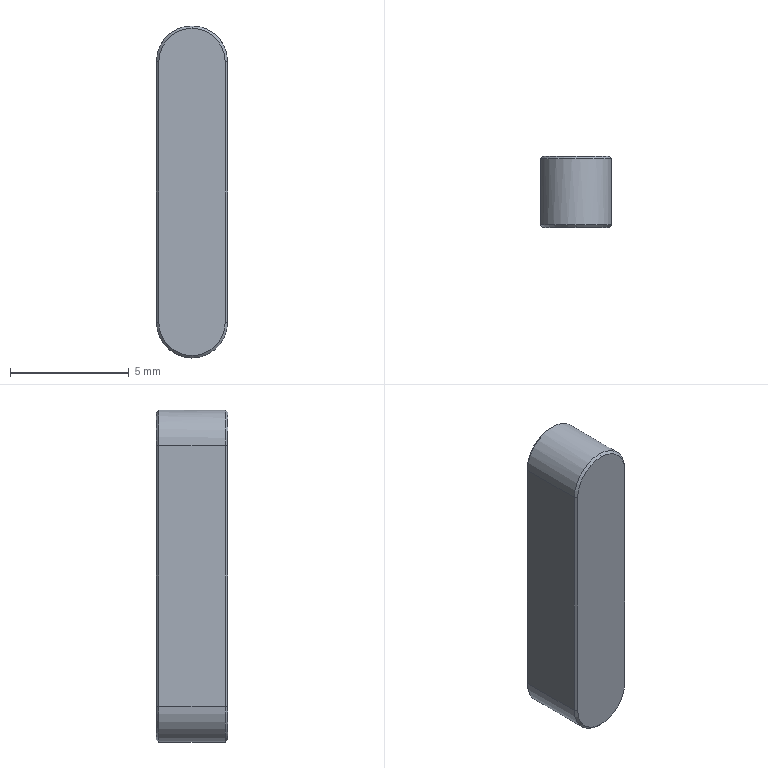Part | STEP file | 1 solid | 17 faces | box 3 x 3 x 14 mm | volume 119.894 mm3 | plane 8 | cone 6 | cylinder 3 | commonest cylinder face diameters 3 x3
STEP:
#1=CARTESIAN_POINT('',(0.,0.,0.));
#2=DIRECTION('',(0.,0.,1.));
#3=DIRECTION('',(1.,0.,0.));
#4=AXIS2_PLACEMENT_3D('',#1,#2,#3);
#5=CARTESIAN_POINT('',(0.,1.5,-6.9));
#6=VERTEX_POINT('',#5);
#7=CARTESIAN_POINT('',(-1.4,1.5,-5.5));
#8=VERTEX_POINT('',#7);
#9=CARTESIAN_POINT('',(0.,1.5,-5.5));
#10=DIRECTION('',(0.,1.,0.));
#11=DIRECTION('',(0.,0.,1.));
#12=AXIS2_PLACEMENT_3D('',#9,#10,#11);
#13=CIRCLE('',#12,1.4);
#14=CARTESIAN_POINT('',(0.,1.5,-5.5));
#15=DIRECTION('',(0.,-1.,0.));
#16=DIRECTION('',(0.,0.,-1.));
#17=AXIS2_PLACEMENT_3D('',#14,#15,#16);
#18=CONICAL_SURFACE('',#17,1.4,0.7854);
#19=CARTESIAN_POINT('',(9.425,0.));
#20=DIRECTION('',(-1.,0.));
#21=VECTOR('',#20,1.);
#22=LINE('',#19,#21);
#23=(GEOMETRIC_REPRESENTATION_CONTEXT(2)PARAMETRIC_REPRESENTATION_CONTEXT()REPRESENTATION_CONTEXT('',''));
#24=DEFINITIONAL_REPRESENTATION('',(#22),#23);
#25=PCURVE('',#18,#24);
#26=CARTESIAN_POINT('',(0.,1.5,5.5));
#27=DIRECTION('',(0.,1.,0.));
#28=DIRECTION('',(0.,0.,1.));
#29=AXIS2_PLACEMENT_3D('',#26,#27,#28);
#30=PLANE('',#29);
#31=CARTESIAN_POINT('',(-11.,0.));
#32=DIRECTION('',(1.,0.));
#33=AXIS2_PLACEMENT_2D('',#31,#32);
#34=CIRCLE('',#33,1.4);
#35=(GEOMETRIC_REPRESENTATION_CONTEXT(2)PARAMETRIC_REPRESENTATION_CONTEXT()REPRESENTATION_CONTEXT('',''));
#36=DEFINITIONAL_REPRESENTATION('',(#34),#35);
#37=PCURVE('',#30,#36);
#38=SURFACE_CURVE('',#13,(#25,#37),.PCURVE_S1.);
#39=EDGE_CURVE('',#6,#8,#38,.T.);
#40=ORIENTED_EDGE('',*,*,#39,.F.);
#41=CARTESIAN_POINT('',(0.,1.4,-7.));
#42=VERTEX_POINT('',#41);
#43=CARTESIAN_POINT('',(0.,1.5,-6.9));
#44=DIRECTION('',(0.,-0.7071,-0.7071));
#45=VECTOR('',#44,1.);
#46=LINE('',#43,#45);
#47=CARTESIAN_POINT('',(6.283,0.));
#48=DIRECTION('',(0.,1.));
#49=VECTOR('',#48,1.);
#50=LINE('',#47,#49);
#51=(GEOMETRIC_REPRESENTATION_CONTEXT(2)PARAMETRIC_REPRESENTATION_CONTEXT()REPRESENTATION_CONTEXT('',''));
#52=DEFINITIONAL_REPRESENTATION('',(#50),#51);
#53=PCURVE('',#18,#52);
#54=CARTESIAN_POINT('',(0.,1.5,-5.5));
#55=DIRECTION('',(0.,-1.,0.));
#56=DIRECTION('',(0.,0.,-1.));
#57=AXIS2_PLACEMENT_3D('',#54,#55,#56);
#58=CONICAL_SURFACE('',#57,1.4,0.7854);
#59=CARTESIAN_POINT('',(0.,0.));
#60=DIRECTION('',(0.,1.));
#61=VECTOR('',#60,1.);
#62=LINE('',#59,#61);
#63=(GEOMETRIC_REPRESENTATION_CONTEXT(2)PARAMETRIC_REPRESENTATION_CONTEXT()REPRESENTATION_CONTEXT('',''));
#64=DEFINITIONAL_REPRESENTATION('',(#62),#63);
#65=PCURVE('',#58,#64);
#66=SURFACE_CURVE('',#46,(#53,#65),.PCURVE_S1.);
#67=EDGE_CURVE('',#6,#42,#66,.T.);
#68=ORIENTED_EDGE('',*,*,#67,.T.);
#69=CARTESIAN_POINT('',(-1.5,1.4,-5.5));
#70=VERTEX_POINT('',#69);
#71=CARTESIAN_POINT('',(0.,1.4,-5.5));
#72=DIRECTION('',(0.,-1.,0.));
#73=DIRECTION('',(0.,0.,1.));
#74=AXIS2_PLACEMENT_3D('',#71,#72,#73);
#75=CIRCLE('',#74,1.5);
#76=CARTESIAN_POINT('',(3.142,0.1));
#77=DIRECTION('',(1.,0.));
#78=VECTOR('',#77,1.);
#79=LINE('',#76,#78);
#80=(GEOMETRIC_REPRESENTATION_CONTEXT(2)PARAMETRIC_REPRESENTATION_CONTEXT()REPRESENTATION_CONTEXT('',''));
#81=DEFINITIONAL_REPRESENTATION('',(#79),#80);
#82=PCURVE('',#18,#81);
#83=CARTESIAN_POINT('',(0.,1.5,-5.5));
#84=DIRECTION('',(0.,-1.,0.));
#85=DIRECTION('',(0.,0.,-1.));
#86=AXIS2_PLACEMENT_3D('',#83,#84,#85);
#87=CYLINDRICAL_SURFACE('',#86,1.5);
#88=CARTESIAN_POINT('',(3.142,0.1));
#89=DIRECTION('',(1.,0.));
#90=VECTOR('',#89,1.);
#91=LINE('',#88,#90);
#92=(GEOMETRIC_REPRESENTATION_CONTEXT(2)PARAMETRIC_REPRESENTATION_CONTEXT()REPRESENTATION_CONTEXT('',''));
#93=DEFINITIONAL_REPRESENTATION('',(#91),#92);
#94=PCURVE('',#87,#93);
#95=SURFACE_CURVE('',#75,(#82,#94),.PCURVE_S1.);
#96=EDGE_CURVE('',#70,#42,#95,.T.);
#97=ORIENTED_EDGE('',*,*,#96,.F.);
#98=CARTESIAN_POINT('',(-1.4,1.5,-5.5));
#99=DIRECTION('',(-0.7071,-0.7071,0.));
#100=VECTOR('',#99,1.);
#101=LINE('',#98,#100);
#102=CARTESIAN_POINT('',(4.712,0.));
#103=DIRECTION('',(0.,1.));
#104=VECTOR('',#103,1.);
#105=LINE('',#102,#104);
#106=(GEOMETRIC_REPRESENTATION_CONTEXT(2)PARAMETRIC_REPRESENTATION_CONTEXT()REPRESENTATION_CONTEXT('',''));
#107=DEFINITIONAL_REPRESENTATION('',(#105),#106);
#108=PCURVE('',#18,#107);
#109=CARTESIAN_POINT('',(-1.4,1.5,5.5));
#110=DIRECTION('',(-0.7071,0.7071,0.));
#111=DIRECTION('',(0.,0.,-1.));
#112=AXIS2_PLACEMENT_3D('',#109,#110,#111);
#113=PLANE('',#112);
#114=CARTESIAN_POINT('',(11.,0.));
#115=DIRECTION('',(0.,1.));
#116=VECTOR('',#115,1.);
#117=LINE('',#114,#116);
#118=(GEOMETRIC_REPRESENTATION_CONTEXT(2)PARAMETRIC_REPRESENTATION_CONTEXT()REPRESENTATION_CONTEXT('',''));
#119=DEFINITIONAL_REPRESENTATION('',(#117),#118);
#120=PCURVE('',#113,#119);
#121=SURFACE_CURVE('',#101,(#108,#120),.PCURVE_S1.);
#122=EDGE_CURVE('',#8,#70,#121,.T.);
#123=ORIENTED_EDGE('',*,*,#122,.F.);
#124=EDGE_LOOP('',(#40,#68,#97,#123));
#125=FACE_BOUND('',#124,.T.);
#126=ADVANCED_FACE('',(#125),#18,.T.);
#127=CARTESIAN_POINT('',(0.,-1.5,6.9));
#128=VERTEX_POINT('',#127);
#129=CARTESIAN_POINT('',(-1.4,-1.5,5.5));
#130=VERTEX_POINT('',#129);
#131=CARTESIAN_POINT('',(0.,-1.5,5.5));
#132=DIRECTION('',(0.,-1.,0.));
#133=DIRECTION('',(0.,0.,1.));
#134=AXIS2_PLACEMENT_3D('',#131,#132,#133);
#135=CIRCLE('',#134,1.4);
#136=CARTESIAN_POINT('',(0.,-1.4,5.5));
#137=DIRECTION('',(0.,1.,0.));
#138=DIRECTION('',(0.,0.,1.));
#139=AXIS2_PLACEMENT_3D('',#136,#137,#138);
#140=CONICAL_SURFACE('',#139,1.5,0.7854);
#141=CARTESIAN_POINT('',(6.283,-0.1));
#142=DIRECTION('',(-1.,0.));
#143=VECTOR('',#142,1.);
#144=LINE('',#141,#143);
#145=(GEOMETRIC_REPRESENTATION_CONTEXT(2)PARAMETRIC_REPRESENTATION_CONTEXT()REPRESENTATION_CONTEXT('',''));
#146=DEFINITIONAL_REPRESENTATION('',(#144),#145);
#147=PCURVE('',#140,#146);
#148=CARTESIAN_POINT('',(0.,-1.5,5.5));
#149=DIRECTION('',(0.,1.,0.));
#150=DIRECTION('',(0.,0.,1.));
#151=AXIS2_PLACEMENT_3D('',#148,#149,#150);
#152=PLANE('',#151);
#153=CARTESIAN_POINT('',(1.4,0.));
#154=CARTESIAN_POINT('',(1.4,-2.425));
#155=CARTESIAN_POINT('',(-0.7,-1.212));
#156=CARTESIAN_POINT('',(-2.8,0.));
#157=CARTESIAN_POINT('',(-0.7,1.212));
#158=CARTESIAN_POINT('',(1.4,2.425));
#159=CARTESIAN_POINT('',(1.4,0.));
#160=(BOUNDED_CURVE()B_SPLINE_CURVE(2,(#153,#154,#155,#156,#157,#158,#159),.UNSPECIFIED.,.T.,.F.)B_SPLINE_CURVE_WITH_KNOTS((1,2,2,2,2,1),(-2.094,0.,2.094,4.189,6.283,8.378),.UNSPECIFIED.)CURVE()GEOMETRIC_REPRESENTATION_ITEM()RATIONAL_B_SPLINE_CURVE((1.,0.5,1.,0.5,1.,0.5,1.))REPRESENTATION_ITEM(''));
#161=(GEOMETRIC_REPRESENTATION_CONTEXT(2)PARAMETRIC_REPRESENTATION_CONTEXT()REPRESENTATION_CONTEXT('',''));
#162=DEFINITIONAL_REPRESENTATION('',(#160),#161);
#163=PCURVE('',#152,#162);
#164=SURFACE_CURVE('',#135,(#147,#163),.PCURVE_S1.);
#165=EDGE_CURVE('',#128,#130,#164,.T.);
#166=ORIENTED_EDGE('',*,*,#165,.F.);
#167=CARTESIAN_POINT('',(0.,-1.4,7.));
#168=VERTEX_POINT('',#167);
#169=CARTESIAN_POINT('',(0.,-1.4,7.));
#170=DIRECTION('',(0.,0.7071,0.7071));
#171=VECTOR('',#170,1.);
#172=LINE('',#169,#171);
#173=CARTESIAN_POINT('',(6.283,0.));
#174=DIRECTION('',(0.,1.));
#175=VECTOR('',#174,1.);
#176=LINE('',#173,#175);
#177=(GEOMETRIC_REPRESENTATION_CONTEXT(2)PARAMETRIC_REPRESENTATION_CONTEXT()REPRESENTATION_CONTEXT('',''));
#178=DEFINITIONAL_REPRESENTATION('',(#176),#177);
#179=PCURVE('',#140,#178);
#180=CARTESIAN_POINT('',(0.,-1.4,5.5));
#181=DIRECTION('',(0.,1.,0.));
#182=DIRECTION('',(0.,0.,1.));
#183=AXIS2_PLACEMENT_3D('',#180,#181,#182);
#184=CONICAL_SURFACE('',#183,1.5,0.7854);
#185=CARTESIAN_POINT('',(0.,0.));
#186=DIRECTION('',(0.,1.));
#187=VECTOR('',#186,1.);
#188=LINE('',#185,#187);
#189=(GEOMETRIC_REPRESENTATION_CONTEXT(2)PARAMETRIC_REPRESENTATION_CONTEXT()REPRESENTATION_CONTEXT('',''));
#190=DEFINITIONAL_REPRESENTATION('',(#188),#189);
#191=PCURVE('',#184,#190);
#192=SURFACE_CURVE('',#172,(#179,#191),.PCURVE_S1.);
#193=EDGE_CURVE('',#128,#168,#192,.T.);
#194=ORIENTED_EDGE('',*,*,#193,.T.);
#195=CARTESIAN_POINT('',(-1.5,-1.4,5.5));
#196=VERTEX_POINT('',#195);
#197=CARTESIAN_POINT('',(0.,-1.4,5.5));
#198=DIRECTION('',(0.,1.,0.));
#199=DIRECTION('',(0.,0.,1.));
#200=AXIS2_PLACEMENT_3D('',#197,#198,#199);
#201=CIRCLE('',#200,1.5);
#202=CARTESIAN_POINT('',(0.,0.));
#203=DIRECTION('',(1.,0.));
#204=VECTOR('',#203,1.);
#205=LINE('',#202,#204);
#206=(GEOMETRIC_REPRESENTATION_CONTEXT(2)PARAMETRIC_REPRESENTATION_CONTEXT()REPRESENTATION_CONTEXT('',''));
#207=DEFINITIONAL_REPRESENTATION('',(#205),#206);
#208=PCURVE('',#140,#207);
#209=CARTESIAN_POINT('',(0.,1.5,5.5));
#210=DIRECTION('',(0.,-1.,0.));
#211=DIRECTION('',(0.,0.,-1.));
#212=AXIS2_PLACEMENT_3D('',#209,#210,#211);
#213=CYLINDRICAL_SURFACE('',#212,1.5);
#214=CARTESIAN_POINT('',(9.425,2.9));
#215=DIRECTION('',(-1.,0.));
#216=VECTOR('',#215,1.);
#217=LINE('',#214,#216);
#218=(GEOMETRIC_REPRESENTATION_CONTEXT(2)PARAMETRIC_REPRESENTATION_CONTEXT()REPRESENTATION_CONTEXT('',''));
#219=DEFINITIONAL_REPRESENTATION('',(#217),#218);
#220=PCURVE('',#213,#219);
#221=SURFACE_CURVE('',#201,(#208,#220),.PCURVE_S1.);
#222=EDGE_CURVE('',#196,#168,#221,.T.);
#223=ORIENTED_EDGE('',*,*,#222,.F.);
#224=CARTESIAN_POINT('',(-1.4,-1.5,5.5));
#225=DIRECTION('',(-0.7071,0.7071,0.));
#226=VECTOR('',#225,1.);
#227=LINE('',#224,#226);
#228=CARTESIAN_POINT('',(4.712,-0.1));
#229=DIRECTION('',(0.,1.));
#230=VECTOR('',#229,1.);
#231=LINE('',#228,#230);
#232=(GEOMETRIC_REPRESENTATION_CONTEXT(2)PARAMETRIC_REPRESENTATION_CONTEXT()REPRESENTATION_CONTEXT('',''));
#233=DEFINITIONAL_REPRESENTATION('',(#231),#232);
#234=PCURVE('',#140,#233);
#235=CARTESIAN_POINT('',(-1.5,-1.4,5.5));
#236=DIRECTION('',(0.7071,0.7071,0.));
#237=DIRECTION('',(0.,0.,1.));
#238=AXIS2_PLACEMENT_3D('',#235,#236,#237);
#239=PLANE('',#238);
#240=CARTESIAN_POINT('',(0.,0.1414));
#241=DIRECTION('',(0.,-1.));
#242=VECTOR('',#241,1.);
#243=LINE('',#240,#242);
#244=(GEOMETRIC_REPRESENTATION_CONTEXT(2)PARAMETRIC_REPRESENTATION_CONTEXT()REPRESENTATION_CONTEXT('',''));
#245=DEFINITIONAL_REPRESENTATION('',(#243),#244);
#246=PCURVE('',#239,#245);
#247=SURFACE_CURVE('',#227,(#234,#246),.PCURVE_S1.);
#248=EDGE_CURVE('',#130,#196,#247,.T.);
#249=ORIENTED_EDGE('',*,*,#248,.F.);
#250=EDGE_LOOP('',(#166,#194,#223,#249));
#251=FACE_BOUND('',#250,.T.);
#252=ADVANCED_FACE('',(#251),#140,.T.);
#253=ORIENTED_EDGE('',*,*,#96,.T.);
#254=CARTESIAN_POINT('',(0.,-1.4,-7.));
#255=VERTEX_POINT('',#254);
#256=CARTESIAN_POINT('',(0.,1.5,-7.));
#257=DIRECTION('',(0.,-1.,0.));
#258=VECTOR('',#257,1.);
#259=LINE('',#256,#258);
#260=CARTESIAN_POINT('',(6.283,0.));
#261=DIRECTION('',(0.,1.));
#262=VECTOR('',#261,1.);
#263=LINE('',#260,#262);
#264=(GEOMETRIC_REPRESENTATION_CONTEXT(2)PARAMETRIC_REPRESENTATION_CONTEXT()REPRESENTATION_CONTEXT('',''));
#265=DEFINITIONAL_REPRESENTATION('',(#263),#264);
#266=PCURVE('',#87,#265);
#267=CARTESIAN_POINT('',(0.,1.5,-5.5));
#268=DIRECTION('',(0.,-1.,0.));
#269=DIRECTION('',(0.,0.,-1.));
#270=AXIS2_PLACEMENT_3D('',#267,#268,#269);
#271=CYLINDRICAL_SURFACE('',#270,1.5);
#272=CARTESIAN_POINT('',(0.,0.));
#273=DIRECTION('',(0.,1.));
#274=VECTOR('',#273,1.);
#275=LINE('',#272,#274);
#276=(GEOMETRIC_REPRESENTATION_CONTEXT(2)PARAMETRIC_REPRESENTATION_CONTEXT()REPRESENTATION_CONTEXT('',''));
#277=DEFINITIONAL_REPRESENTATION('',(#275),#276);
#278=PCURVE('',#271,#277);
#279=SURFACE_CURVE('',#259,(#266,#278),.PCURVE_S1.);
#280=EDGE_CURVE('',#42,#255,#279,.T.);
#281=ORIENTED_EDGE('',*,*,#280,.T.);
#282=CARTESIAN_POINT('',(-1.5,-1.4,-5.5));
#283=VERTEX_POINT('',#282);
#284=CARTESIAN_POINT('',(0.,-1.4,-5.5));
#285=DIRECTION('',(0.,1.,0.));
#286=DIRECTION('',(0.,0.,1.));
#287=AXIS2_PLACEMENT_3D('',#284,#285,#286);
#288=CIRCLE('',#287,1.5);
#289=CARTESIAN_POINT('',(9.425,2.9));
#290=DIRECTION('',(-1.,0.));
#291=VECTOR('',#290,1.);
#292=LINE('',#289,#291);
#293=(GEOMETRIC_REPRESENTATION_CONTEXT(2)PARAMETRIC_REPRESENTATION_CONTEXT()REPRESENTATION_CONTEXT('',''));
#294=DEFINITIONAL_REPRESENTATION('',(#292),#293);
#295=PCURVE('',#87,#294);
#296=CARTESIAN_POINT('',(0.,-1.4,-5.5));
#297=DIRECTION('',(0.,1.,0.));
#298=DIRECTION('',(0.,0.,1.));
#299=AXIS2_PLACEMENT_3D('',#296,#297,#298);
#300=CONICAL_SURFACE('',#299,1.5,0.7854);
#301=CARTESIAN_POINT('',(0.,0.));
#302=DIRECTION('',(1.,0.));
#303=VECTOR('',#302,1.);
#304=LINE('',#301,#303);
#305=(GEOMETRIC_REPRESENTATION_CONTEXT(2)PARAMETRIC_REPRESENTATION_CONTEXT()REPRESENTATION_CONTEXT('',''));
#306=DEFINITIONAL_REPRESENTATION('',(#304),#305);
#307=PCURVE('',#300,#306);
#308=SURFACE_CURVE('',#288,(#295,#307),.PCURVE_S1.);
#309=EDGE_CURVE('',#255,#283,#308,.T.);
#310=ORIENTED_EDGE('',*,*,#309,.T.);
#311=CARTESIAN_POINT('',(-1.5,1.5,-5.5));
#312=DIRECTION('',(0.,-1.,0.));
#313=VECTOR('',#312,1.);
#314=LINE('',#311,#313);
#315=CARTESIAN_POINT('',(4.712,0.));
#316=DIRECTION('',(0.,1.));
#317=VECTOR('',#316,1.);
#318=LINE('',#315,#317);
#319=(GEOMETRIC_REPRESENTATION_CONTEXT(2)PARAMETRIC_REPRESENTATION_CONTEXT()REPRESENTATION_CONTEXT('',''));
#320=DEFINITIONAL_REPRESENTATION('',(#318),#319);
#321=PCURVE('',#87,#320);
#322=CARTESIAN_POINT('',(-1.5,1.5,5.5));
#323=DIRECTION('',(1.,0.,0.));
#324=DIRECTION('',(0.,0.,-1.));
#325=AXIS2_PLACEMENT_3D('',#322,#323,#324);
#326=PLANE('',#325);
#327=CARTESIAN_POINT('',(11.,0.));
#328=DIRECTION('',(0.,-1.));
#329=VECTOR('',#328,1.);
#330=LINE('',#327,#329);
#331=(GEOMETRIC_REPRESENTATION_CONTEXT(2)PARAMETRIC_REPRESENTATION_CONTEXT()REPRESENTATION_CONTEXT('',''));
#332=DEFINITIONAL_REPRESENTATION('',(#330),#331);
#333=PCURVE('',#326,#332);
#334=SURFACE_CURVE('',#314,(#321,#333),.PCURVE_S1.);
#335=EDGE_CURVE('',#70,#283,#334,.T.);
#336=ORIENTED_EDGE('',*,*,#335,.F.);
#337=EDGE_LOOP('',(#253,#281,#310,#336));
#338=FACE_BOUND('',#337,.T.);
#339=ADVANCED_FACE('',(#338),#87,.T.);
#340=CARTESIAN_POINT('',(-1.5,1.4,5.5));
#341=VERTEX_POINT('',#340);
#342=CARTESIAN_POINT('',(-1.5,1.5,5.5));
#343=DIRECTION('',(0.,-1.,0.));
#344=VECTOR('',#343,1.);
#345=LINE('',#342,#344);
#346=CARTESIAN_POINT('',(4.712,0.));
#347=DIRECTION('',(0.,1.));
#348=VECTOR('',#347,1.);
#349=LINE('',#346,#348);
#350=(GEOMETRIC_REPRESENTATION_CONTEXT(2)PARAMETRIC_REPRESENTATION_CONTEXT()REPRESENTATION_CONTEXT('',''));
#351=DEFINITIONAL_REPRESENTATION('',(#349),#350);
#352=PCURVE('',#213,#351);
#353=CARTESIAN_POINT('',(0.,0.));
#354=DIRECTION('',(0.,-1.));
#355=VECTOR('',#354,1.);
#356=LINE('',#353,#355);
#357=(GEOMETRIC_REPRESENTATION_CONTEXT(2)PARAMETRIC_REPRESENTATION_CONTEXT()REPRESENTATION_CONTEXT('',''));
#358=DEFINITIONAL_REPRESENTATION('',(#356),#357);
#359=PCURVE('',#326,#358);
#360=SURFACE_CURVE('',#345,(#352,#359),.PCURVE_S1.);
#361=EDGE_CURVE('',#341,#196,#360,.T.);
#362=ORIENTED_EDGE('',*,*,#361,.T.);
#363=ORIENTED_EDGE('',*,*,#222,.T.);
#364=CARTESIAN_POINT('',(1.5,-1.4,5.5));
#365=VERTEX_POINT('',#364);
#366=CARTESIAN_POINT('',(0.,-1.4,5.5));
#367=DIRECTION('',(0.,1.,0.));
#368=DIRECTION('',(0.,0.,1.));
#369=AXIS2_PLACEMENT_3D('',#366,#367,#368);
#370=CIRCLE('',#369,1.5);
#371=CARTESIAN_POINT('',(3.142,2.9));
#372=DIRECTION('',(-1.,0.));
#373=VECTOR('',#372,1.);
#374=LINE('',#371,#373);
#375=(GEOMETRIC_REPRESENTATION_CONTEXT(2)PARAMETRIC_REPRESENTATION_CONTEXT()REPRESENTATION_CONTEXT('',''));
#376=DEFINITIONAL_REPRESENTATION('',(#374),#375);
#377=PCURVE('',#213,#376);
#378=CARTESIAN_POINT('',(0.,0.));
#379=DIRECTION('',(1.,0.));
#380=VECTOR('',#379,1.);
#381=LINE('',#378,#380);
#382=(GEOMETRIC_REPRESENTATION_CONTEXT(2)PARAMETRIC_REPRESENTATION_CONTEXT()REPRESENTATION_CONTEXT('',''));
#383=DEFINITIONAL_REPRESENTATION('',(#381),#382);
#384=PCURVE('',#184,#383);
#385=SURFACE_CURVE('',#370,(#377,#384),.PCURVE_S1.);
#386=EDGE_CURVE('',#168,#365,#385,.T.);
#387=ORIENTED_EDGE('',*,*,#386,.T.);
#388=CARTESIAN_POINT('',(1.5,1.4,5.5));
#389=VERTEX_POINT('',#388);
#390=CARTESIAN_POINT('',(1.5,1.5,5.5));
#391=DIRECTION('',(0.,-1.,0.));
#392=VECTOR('',#391,1.);
#393=LINE('',#390,#392);
#394=CARTESIAN_POINT('',(1.571,0.));
#395=DIRECTION('',(0.,1.));
#396=VECTOR('',#395,1.);
#397=LINE('',#394,#396);
#398=(GEOMETRIC_REPRESENTATION_CONTEXT(2)PARAMETRIC_REPRESENTATION_CONTEXT()REPRESENTATION_CONTEXT('',''));
#399=DEFINITIONAL_REPRESENTATION('',(#397),#398);
#400=PCURVE('',#213,#399);
#401=CARTESIAN_POINT('',(1.5,1.5,5.5));
#402=DIRECTION('',(-1.,0.,0.));
#403=DIRECTION('',(0.,0.,1.));
#404=AXIS2_PLACEMENT_3D('',#401,#402,#403);
#405=PLANE('',#404);
#406=CARTESIAN_POINT('',(0.,0.));
#407=DIRECTION('',(0.,-1.));
#408=VECTOR('',#407,1.);
#409=LINE('',#406,#408);
#410=(GEOMETRIC_REPRESENTATION_CONTEXT(2)PARAMETRIC_REPRESENTATION_CONTEXT()REPRESENTATION_CONTEXT('',''));
#411=DEFINITIONAL_REPRESENTATION('',(#409),#410);
#412=PCURVE('',#405,#411);
#413=SURFACE_CURVE('',#393,(#400,#412),.PCURVE_S1.);
#414=EDGE_CURVE('',#389,#365,#413,.T.);
#415=ORIENTED_EDGE('',*,*,#414,.F.);
#416=CARTESIAN_POINT('',(0.,1.4,5.5));
#417=DIRECTION('',(0.,-1.,0.));
#418=DIRECTION('',(0.,0.,1.));
#419=AXIS2_PLACEMENT_3D('',#416,#417,#418);
#420=CIRCLE('',#419,1.5);
#421=CARTESIAN_POINT('',(-3.142,0.1));
#422=DIRECTION('',(1.,0.));
#423=VECTOR('',#422,1.);
#424=LINE('',#421,#423);
#425=(GEOMETRIC_REPRESENTATION_CONTEXT(2)PARAMETRIC_REPRESENTATION_CONTEXT()REPRESENTATION_CONTEXT('',''));
#426=DEFINITIONAL_REPRESENTATION('',(#424),#425);
#427=PCURVE('',#213,#426);
#428=CARTESIAN_POINT('',(0.,1.5,5.5));
#429=DIRECTION('',(0.,-1.,0.));
#430=DIRECTION('',(0.,0.,-1.));
#431=AXIS2_PLACEMENT_3D('',#428,#429,#430);
#432=CONICAL_SURFACE('',#431,1.4,0.7854);
#433=CARTESIAN_POINT('',(-3.142,0.1));
#434=DIRECTION('',(1.,0.));
#435=VECTOR('',#434,1.);
#436=LINE('',#433,#435);
#437=(GEOMETRIC_REPRESENTATION_CONTEXT(2)PARAMETRIC_REPRESENTATION_CONTEXT()REPRESENTATION_CONTEXT('',''));
#438=DEFINITIONAL_REPRESENTATION('',(#436),#437);
#439=PCURVE('',#432,#438);
#440=SURFACE_CURVE('',#420,(#427,#439),.PCURVE_S1.);
#441=EDGE_CURVE('',#389,#341,#440,.T.);
#442=ORIENTED_EDGE('',*,*,#441,.T.);
#443=EDGE_LOOP('',(#362,#363,#387,#415,#442));
#444=FACE_BOUND('',#443,.T.);
#445=ADVANCED_FACE('',(#444),#213,.T.);
#446=ORIENTED_EDGE('',*,*,#414,.T.);
#447=CARTESIAN_POINT('',(1.5,-1.4,-5.5));
#448=VERTEX_POINT('',#447);
#449=CARTESIAN_POINT('',(1.5,-1.4,5.5));
#450=DIRECTION('',(0.,0.,-1.));
#451=VECTOR('',#450,1.);
#452=LINE('',#449,#451);
#453=CARTESIAN_POINT('',(0.,-2.9));
#454=DIRECTION('',(-1.,0.));
#455=VECTOR('',#454,1.);
#456=LINE('',#453,#455);
#457=(GEOMETRIC_REPRESENTATION_CONTEXT(2)PARAMETRIC_REPRESENTATION_CONTEXT()REPRESENTATION_CONTEXT('',''));
#458=DEFINITIONAL_REPRESENTATION('',(#456),#457);
#459=PCURVE('',#405,#458);
#460=CARTESIAN_POINT('',(1.5,-1.4,5.5));
#461=DIRECTION('',(-0.7071,0.7071,0.));
#462=DIRECTION('',(0.,0.,-1.));
#463=AXIS2_PLACEMENT_3D('',#460,#461,#462);
#464=PLANE('',#463);
#465=CARTESIAN_POINT('',(0.,0.));
#466=DIRECTION('',(1.,0.));
#467=VECTOR('',#466,1.);
#468=LINE('',#465,#467);
#469=(GEOMETRIC_REPRESENTATION_CONTEXT(2)PARAMETRIC_REPRESENTATION_CONTEXT()REPRESENTATION_CONTEXT('',''));
#470=DEFINITIONAL_REPRESENTATION('',(#468),#469);
#471=PCURVE('',#464,#470);
#472=SURFACE_CURVE('',#452,(#459,#471),.PCURVE_S1.);
#473=EDGE_CURVE('',#365,#448,#472,.T.);
#474=ORIENTED_EDGE('',*,*,#473,.T.);
#475=CARTESIAN_POINT('',(1.5,1.4,-5.5));
#476=VERTEX_POINT('',#475);
#477=CARTESIAN_POINT('',(1.5,1.5,-5.5));
#478=DIRECTION('',(0.,-1.,0.));
#479=VECTOR('',#478,1.);
#480=LINE('',#477,#479);
#481=CARTESIAN_POINT('',(-11.,0.));
#482=DIRECTION('',(0.,-1.));
#483=VECTOR('',#482,1.);
#484=LINE('',#481,#483);
#485=(GEOMETRIC_REPRESENTATION_CONTEXT(2)PARAMETRIC_REPRESENTATION_CONTEXT()REPRESENTATION_CONTEXT('',''));
#486=DEFINITIONAL_REPRESENTATION('',(#484),#485);
#487=PCURVE('',#405,#486);
#488=CARTESIAN_POINT('',(1.571,0.));
#489=DIRECTION('',(0.,1.));
#490=VECTOR('',#489,1.);
#491=LINE('',#488,#490);
#492=(GEOMETRIC_REPRESENTATION_CONTEXT(2)PARAMETRIC_REPRESENTATION_CONTEXT()REPRESENTATION_CONTEXT('',''));
#493=DEFINITIONAL_REPRESENTATION('',(#491),#492);
#494=PCURVE('',#271,#493);
#495=SURFACE_CURVE('',#480,(#487,#494),.PCURVE_S1.);
#496=EDGE_CURVE('',#476,#448,#495,.T.);
#497=ORIENTED_EDGE('',*,*,#496,.F.);
#498=CARTESIAN_POINT('',(1.5,1.4,5.5));
#499=DIRECTION('',(0.,0.,1.));
#500=VECTOR('',#499,1.);
#501=LINE('',#498,#500);
#502=CARTESIAN_POINT('',(0.,-0.1));
#503=DIRECTION('',(1.,0.));
#504=VECTOR('',#503,1.);
#505=LINE('',#502,#504);
#506=(GEOMETRIC_REPRESENTATION_CONTEXT(2)PARAMETRIC_REPRESENTATION_CONTEXT()REPRESENTATION_CONTEXT('',''));
#507=DEFINITIONAL_REPRESENTATION('',(#505),#506);
#508=PCURVE('',#405,#507);
#509=CARTESIAN_POINT('',(1.4,1.5,5.5));
#510=DIRECTION('',(0.7071,0.7071,0.));
#511=DIRECTION('',(0.,0.,1.));
#512=AXIS2_PLACEMENT_3D('',#509,#510,#511);
#513=PLANE('',#512);
#514=CARTESIAN_POINT('',(0.,0.1414));
#515=DIRECTION('',(1.,0.));
#516=VECTOR('',#515,1.);
#517=LINE('',#514,#516);
#518=(GEOMETRIC_REPRESENTATION_CONTEXT(2)PARAMETRIC_REPRESENTATION_CONTEXT()REPRESENTATION_CONTEXT('',''));
#519=DEFINITIONAL_REPRESENTATION('',(#517),#518);
#520=PCURVE('',#513,#519);
#521=SURFACE_CURVE('',#501,(#508,#520),.PCURVE_S1.);
#522=EDGE_CURVE('',#476,#389,#521,.T.);
#523=ORIENTED_EDGE('',*,*,#522,.T.);
#524=EDGE_LOOP('',(#446,#474,#497,#523));
#525=FACE_BOUND('',#524,.T.);
#526=ADVANCED_FACE('',(#525),#405,.F.);
#527=ORIENTED_EDGE('',*,*,#280,.F.);
#528=CARTESIAN_POINT('',(0.,1.4,-5.5));
#529=DIRECTION('',(0.,-1.,0.));
#530=DIRECTION('',(0.,0.,1.));
#531=AXIS2_PLACEMENT_3D('',#528,#529,#530);
#532=CIRCLE('',#531,1.5);
#533=CARTESIAN_POINT('',(-3.142,0.1));
#534=DIRECTION('',(1.,0.));
#535=VECTOR('',#534,1.);
#536=LINE('',#533,#535);
#537=(GEOMETRIC_REPRESENTATION_CONTEXT(2)PARAMETRIC_REPRESENTATION_CONTEXT()REPRESENTATION_CONTEXT('',''));
#538=DEFINITIONAL_REPRESENTATION('',(#536),#537);
#539=PCURVE('',#271,#538);
#540=CARTESIAN_POINT('',(-3.142,0.1));
#541=DIRECTION('',(1.,0.));
#542=VECTOR('',#541,1.);
#543=LINE('',#540,#542);
#544=(GEOMETRIC_REPRESENTATION_CONTEXT(2)PARAMETRIC_REPRESENTATION_CONTEXT()REPRESENTATION_CONTEXT('',''));
#545=DEFINITIONAL_REPRESENTATION('',(#543),#544);
#546=PCURVE('',#58,#545);
#547=SURFACE_CURVE('',#532,(#539,#546),.PCURVE_S1.);
#548=EDGE_CURVE('',#42,#476,#547,.T.);
#549=ORIENTED_EDGE('',*,*,#548,.T.);
#550=ORIENTED_EDGE('',*,*,#496,.T.);
#551=CARTESIAN_POINT('',(0.,-1.4,-5.5));
#552=DIRECTION('',(0.,1.,0.));
#553=DIRECTION('',(0.,0.,1.));
#554=AXIS2_PLACEMENT_3D('',#551,#552,#553);
#555=CIRCLE('',#554,1.5);
#556=CARTESIAN_POINT('',(3.142,2.9));
#557=DIRECTION('',(-1.,0.));
#558=VECTOR('',#557,1.);
#559=LINE('',#556,#558);
#560=(GEOMETRIC_REPRESENTATION_CONTEXT(2)PARAMETRIC_REPRESENTATION_CONTEXT()REPRESENTATION_CONTEXT('',''));
#561=DEFINITIONAL_REPRESENTATION('',(#559),#560);
#562=PCURVE('',#271,#561);
#563=CARTESIAN_POINT('',(0.,0.));
#564=DIRECTION('',(1.,0.));
#565=VECTOR('',#564,1.);
#566=LINE('',#563,#565);
#567=(GEOMETRIC_REPRESENTATION_CONTEXT(2)PARAMETRIC_REPRESENTATION_CONTEXT()REPRESENTATION_CONTEXT('',''));
#568=DEFINITIONAL_REPRESENTATION('',(#566),#567);
#569=PCURVE('',#300,#568);
#570=SURFACE_CURVE('',#555,(#562,#569),.PCURVE_S1.);
#571=EDGE_CURVE('',#448,#255,#570,.T.);
#572=ORIENTED_EDGE('',*,*,#571,.T.);
#573=EDGE_LOOP('',(#527,#549,#550,#572));
#574=FACE_BOUND('',#573,.T.);
#575=ADVANCED_FACE('',(#574),#271,.T.);
#576=ORIENTED_EDGE('',*,*,#335,.T.);
#577=CARTESIAN_POINT('',(-1.5,-1.4,5.5));
#578=DIRECTION('',(0.,0.,1.));
#579=VECTOR('',#578,1.);
#580=LINE('',#577,#579);
#581=CARTESIAN_POINT('',(0.,-2.9));
#582=DIRECTION('',(-1.,0.));
#583=VECTOR('',#582,1.);
#584=LINE('',#581,#583);
#585=(GEOMETRIC_REPRESENTATION_CONTEXT(2)PARAMETRIC_REPRESENTATION_CONTEXT()REPRESENTATION_CONTEXT('',''));
#586=DEFINITIONAL_REPRESENTATION('',(#584),#585);
#587=PCURVE('',#326,#586);
#588=CARTESIAN_POINT('',(0.,0.));
#589=DIRECTION('',(1.,0.));
#590=VECTOR('',#589,1.);
#591=LINE('',#588,#590);
#592=(GEOMETRIC_REPRESENTATION_CONTEXT(2)PARAMETRIC_REPRESENTATION_CONTEXT()REPRESENTATION_CONTEXT('',''));
#593=DEFINITIONAL_REPRESENTATION('',(#591),#592);
#594=PCURVE('',#239,#593);
#595=SURFACE_CURVE('',#580,(#587,#594),.PCURVE_S1.);
#596=EDGE_CURVE('',#283,#196,#595,.T.);
#597=ORIENTED_EDGE('',*,*,#596,.T.);
#598=ORIENTED_EDGE('',*,*,#361,.F.);
#599=CARTESIAN_POINT('',(-1.5,1.4,-5.5));
#600=DIRECTION('',(0.,0.,-1.));
#601=VECTOR('',#600,1.);
#602=LINE('',#599,#601);
#603=CARTESIAN_POINT('',(11.,-0.1));
#604=DIRECTION('',(1.,0.));
#605=VECTOR('',#604,1.);
#606=LINE('',#603,#605);
#607=(GEOMETRIC_REPRESENTATION_CONTEXT(2)PARAMETRIC_REPRESENTATION_CONTEXT()REPRESENTATION_CONTEXT('',''));
#608=DEFINITIONAL_REPRESENTATION('',(#606),#607);
#609=PCURVE('',#326,#608);
#610=CARTESIAN_POINT('',(11.,0.1414));
#611=DIRECTION('',(1.,0.));
#612=VECTOR('',#611,1.);
#613=LINE('',#610,#612);
#614=(GEOMETRIC_REPRESENTATION_CONTEXT(2)PARAMETRIC_REPRESENTATION_CONTEXT()REPRESENTATION_CONTEXT('',''));
#615=DEFINITIONAL_REPRESENTATION('',(#613),#614);
#616=PCURVE('',#113,#615);
#617=SURFACE_CURVE('',#602,(#609,#616),.PCURVE_S1.);
#618=EDGE_CURVE('',#341,#70,#617,.T.);
#619=ORIENTED_EDGE('',*,*,#618,.T.);
#620=EDGE_LOOP('',(#576,#597,#598,#619));
#621=FACE_BOUND('',#620,.T.);
#622=ADVANCED_FACE('',(#621),#326,.F.);
#623=CARTESIAN_POINT('',(1.4,1.5,-5.5));
#624=VERTEX_POINT('',#623);
#625=CARTESIAN_POINT('',(0.,1.5,-5.5));
#626=DIRECTION('',(0.,1.,0.));
#627=DIRECTION('',(0.,0.,1.));
#628=AXIS2_PLACEMENT_3D('',#625,#626,#627);
#629=CIRCLE('',#628,1.4);
#630=CARTESIAN_POINT('',(-11.,0.));
#631=DIRECTION('',(1.,0.));
#632=AXIS2_PLACEMENT_2D('',#630,#631);
#633=CIRCLE('',#632,1.4);
#634=(GEOMETRIC_REPRESENTATION_CONTEXT(2)PARAMETRIC_REPRESENTATION_CONTEXT()REPRESENTATION_CONTEXT('',''));
#635=DEFINITIONAL_REPRESENTATION('',(#633),#634);
#636=PCURVE('',#30,#635);
#637=CARTESIAN_POINT('',(3.142,0.));
#638=DIRECTION('',(-1.,0.));
#639=VECTOR('',#638,1.);
#640=LINE('',#637,#639);
#641=(GEOMETRIC_REPRESENTATION_CONTEXT(2)PARAMETRIC_REPRESENTATION_CONTEXT()REPRESENTATION_CONTEXT('',''));
#642=DEFINITIONAL_REPRESENTATION('',(#640),#641);
#643=PCURVE('',#58,#642);
#644=SURFACE_CURVE('',#629,(#636,#643),.PCURVE_S1.);
#645=EDGE_CURVE('',#624,#6,#644,.T.);
#646=ORIENTED_EDGE('',*,*,#645,.T.);
#647=ORIENTED_EDGE('',*,*,#39,.T.);
#648=CARTESIAN_POINT('',(-1.4,1.5,5.5));
#649=VERTEX_POINT('',#648);
#650=CARTESIAN_POINT('',(-1.4,1.5,5.5));
#651=DIRECTION('',(0.,0.,1.));
#652=VECTOR('',#651,1.);
#653=LINE('',#650,#652);
#654=CARTESIAN_POINT('',(0.,-1.4));
#655=DIRECTION('',(1.,0.));
#656=VECTOR('',#655,1.);
#657=LINE('',#654,#656);
#658=(GEOMETRIC_REPRESENTATION_CONTEXT(2)PARAMETRIC_REPRESENTATION_CONTEXT()REPRESENTATION_CONTEXT('',''));
#659=DEFINITIONAL_REPRESENTATION('',(#657),#658);
#660=PCURVE('',#30,#659);
#661=CARTESIAN_POINT('',(0.,0.));
#662=DIRECTION('',(-1.,0.));
#663=VECTOR('',#662,1.);
#664=LINE('',#661,#663);
#665=(GEOMETRIC_REPRESENTATION_CONTEXT(2)PARAMETRIC_REPRESENTATION_CONTEXT()REPRESENTATION_CONTEXT('',''));
#666=DEFINITIONAL_REPRESENTATION('',(#664),#665);
#667=PCURVE('',#113,#666);
#668=SURFACE_CURVE('',#653,(#660,#667),.PCURVE_S1.);
#669=EDGE_CURVE('',#8,#649,#668,.T.);
#670=ORIENTED_EDGE('',*,*,#669,.T.);
#671=CARTESIAN_POINT('',(1.4,1.5,5.5));
#672=VERTEX_POINT('',#671);
#673=CARTESIAN_POINT('',(0.,1.5,5.5));
#674=DIRECTION('',(0.,1.,0.));
#675=DIRECTION('',(0.,0.,1.));
#676=AXIS2_PLACEMENT_3D('',#673,#674,#675);
#677=CIRCLE('',#676,1.4);
#678=CARTESIAN_POINT('',(0.,0.));
#679=DIRECTION('',(1.,0.));
#680=AXIS2_PLACEMENT_2D('',#678,#679);
#681=CIRCLE('',#680,1.4);
#682=(GEOMETRIC_REPRESENTATION_CONTEXT(2)PARAMETRIC_REPRESENTATION_CONTEXT()REPRESENTATION_CONTEXT('',''));
#683=DEFINITIONAL_REPRESENTATION('',(#681),#682);
#684=PCURVE('',#30,#683);
#685=CARTESIAN_POINT('',(9.425,0.));
#686=DIRECTION('',(-1.,0.));
#687=VECTOR('',#686,1.);
#688=LINE('',#685,#687);
#689=(GEOMETRIC_REPRESENTATION_CONTEXT(2)PARAMETRIC_REPRESENTATION_CONTEXT()REPRESENTATION_CONTEXT('',''));
#690=DEFINITIONAL_REPRESENTATION('',(#688),#689);
#691=PCURVE('',#432,#690);
#692=SURFACE_CURVE('',#677,(#684,#691),.PCURVE_S1.);
#693=EDGE_CURVE('',#649,#672,#692,.T.);
#694=ORIENTED_EDGE('',*,*,#693,.T.);
#695=CARTESIAN_POINT('',(1.4,1.5,-5.5));
#696=DIRECTION('',(0.,0.,-1.));
#697=VECTOR('',#696,1.);
#698=LINE('',#695,#697);
#699=CARTESIAN_POINT('',(-11.,1.4));
#700=DIRECTION('',(-1.,0.));
#701=VECTOR('',#700,1.);
#702=LINE('',#699,#701);
#703=(GEOMETRIC_REPRESENTATION_CONTEXT(2)PARAMETRIC_REPRESENTATION_CONTEXT()REPRESENTATION_CONTEXT('',''));
#704=DEFINITIONAL_REPRESENTATION('',(#702),#703);
#705=PCURVE('',#30,#704);
#706=CARTESIAN_POINT('',(-11.,0.));
#707=DIRECTION('',(-1.,0.));
#708=VECTOR('',#707,1.);
#709=LINE('',#706,#708);
#710=(GEOMETRIC_REPRESENTATION_CONTEXT(2)PARAMETRIC_REPRESENTATION_CONTEXT()REPRESENTATION_CONTEXT('',''));
#711=DEFINITIONAL_REPRESENTATION('',(#709),#710);
#712=PCURVE('',#513,#711);
#713=SURFACE_CURVE('',#698,(#705,#712),.PCURVE_S1.);
#714=EDGE_CURVE('',#672,#624,#713,.T.);
#715=ORIENTED_EDGE('',*,*,#714,.T.);
#716=EDGE_LOOP('',(#646,#647,#670,#694,#715));
#717=FACE_BOUND('',#716,.T.);
#718=ADVANCED_FACE('',(#717),#30,.T.);
#719=CARTESIAN_POINT('',(1.4,-1.5,5.5));
#720=VERTEX_POINT('',#719);
#721=CARTESIAN_POINT('',(0.,-1.5,5.5));
#722=DIRECTION('',(0.,-1.,0.));
#723=DIRECTION('',(0.,0.,1.));
#724=AXIS2_PLACEMENT_3D('',#721,#722,#723);
#725=CIRCLE('',#724,1.4);
#726=CARTESIAN_POINT('',(1.4,0.));
#727=CARTESIAN_POINT('',(1.4,-2.425));
#728=CARTESIAN_POINT('',(-0.7,-1.212));
#729=CARTESIAN_POINT('',(-2.8,0.));
#730=CARTESIAN_POINT('',(-0.7,1.212));
#731=CARTESIAN_POINT('',(1.4,2.425));
#732=CARTESIAN_POINT('',(1.4,0.));
#733=(BOUNDED_CURVE()B_SPLINE_CURVE(2,(#726,#727,#728,#729,#730,#731,#732),.UNSPECIFIED.,.T.,.F.)B_SPLINE_CURVE_WITH_KNOTS((1,2,2,2,2,1),(-2.094,0.,2.094,4.189,6.283,8.378),.UNSPECIFIED.)CURVE()GEOMETRIC_REPRESENTATION_ITEM()RATIONAL_B_SPLINE_CURVE((1.,0.5,1.,0.5,1.,0.5,1.))REPRESENTATION_ITEM(''));
#734=(GEOMETRIC_REPRESENTATION_CONTEXT(2)PARAMETRIC_REPRESENTATION_CONTEXT()REPRESENTATION_CONTEXT('',''));
#735=DEFINITIONAL_REPRESENTATION('',(#733),#734);
#736=PCURVE('',#152,#735);
#737=CARTESIAN_POINT('',(6.283,-0.1));
#738=DIRECTION('',(-1.,0.));
#739=VECTOR('',#738,1.);
#740=LINE('',#737,#739);
#741=(GEOMETRIC_REPRESENTATION_CONTEXT(2)PARAMETRIC_REPRESENTATION_CONTEXT()REPRESENTATION_CONTEXT('',''));
#742=DEFINITIONAL_REPRESENTATION('',(#740),#741);
#743=PCURVE('',#184,#742);
#744=SURFACE_CURVE('',#725,(#736,#743),.PCURVE_S1.);
#745=EDGE_CURVE('',#720,#128,#744,.T.);
#746=ORIENTED_EDGE('',*,*,#745,.T.);
#747=ORIENTED_EDGE('',*,*,#165,.T.);
#748=CARTESIAN_POINT('',(-1.4,-1.5,-5.5));
#749=VERTEX_POINT('',#748);
#750=CARTESIAN_POINT('',(-1.4,-1.5,5.5));
#751=DIRECTION('',(0.,0.,-1.));
#752=VECTOR('',#751,1.);
#753=LINE('',#750,#752);
#754=CARTESIAN_POINT('',(0.,-1.4));
#755=DIRECTION('',(-1.,0.));
#756=VECTOR('',#755,1.);
#757=LINE('',#754,#756);
#758=(GEOMETRIC_REPRESENTATION_CONTEXT(2)PARAMETRIC_REPRESENTATION_CONTEXT()REPRESENTATION_CONTEXT('',''));
#759=DEFINITIONAL_REPRESENTATION('',(#757),#758);
#760=PCURVE('',#152,#759);
#761=CARTESIAN_POINT('',(0.,0.1414));
#762=DIRECTION('',(-1.,0.));
#763=VECTOR('',#762,1.);
#764=LINE('',#761,#763);
#765=(GEOMETRIC_REPRESENTATION_CONTEXT(2)PARAMETRIC_REPRESENTATION_CONTEXT()REPRESENTATION_CONTEXT('',''));
#766=DEFINITIONAL_REPRESENTATION('',(#764),#765);
#767=PCURVE('',#239,#766);
#768=SURFACE_CURVE('',#753,(#760,#767),.PCURVE_S1.);
#769=EDGE_CURVE('',#130,#749,#768,.T.);
#770=ORIENTED_EDGE('',*,*,#769,.T.);
#771=CARTESIAN_POINT('',(1.4,-1.5,-5.5));
#772=VERTEX_POINT('',#771);
#773=CARTESIAN_POINT('',(0.,-1.5,-5.5));
#774=DIRECTION('',(0.,-1.,0.));
#775=DIRECTION('',(0.,0.,1.));
#776=AXIS2_PLACEMENT_3D('',#773,#774,#775);
#777=CIRCLE('',#776,1.4);
#778=CARTESIAN_POINT('',(-9.6,0.));
#779=CARTESIAN_POINT('',(-9.6,-2.425));
#780=CARTESIAN_POINT('',(-11.7,-1.212));
#781=CARTESIAN_POINT('',(-13.8,0.));
#782=CARTESIAN_POINT('',(-11.7,1.212));
#783=CARTESIAN_POINT('',(-9.6,2.425));
#784=CARTESIAN_POINT('',(-9.6,0.));
#785=(BOUNDED_CURVE()B_SPLINE_CURVE(2,(#778,#779,#780,#781,#782,#783,#784),.UNSPECIFIED.,.T.,.F.)B_SPLINE_CURVE_WITH_KNOTS((1,2,2,2,2,1),(-2.094,0.,2.094,4.189,6.283,8.378),.UNSPECIFIED.)CURVE()GEOMETRIC_REPRESENTATION_ITEM()RATIONAL_B_SPLINE_CURVE((1.,0.5,1.,0.5,1.,0.5,1.))REPRESENTATION_ITEM(''));
#786=(GEOMETRIC_REPRESENTATION_CONTEXT(2)PARAMETRIC_REPRESENTATION_CONTEXT()REPRESENTATION_CONTEXT('',''));
#787=DEFINITIONAL_REPRESENTATION('',(#785),#786);
#788=PCURVE('',#152,#787);
#789=CARTESIAN_POINT('',(6.283,-0.1));
#790=DIRECTION('',(-1.,0.));
#791=VECTOR('',#790,1.);
#792=LINE('',#789,#791);
#793=(GEOMETRIC_REPRESENTATION_CONTEXT(2)PARAMETRIC_REPRESENTATION_CONTEXT()REPRESENTATION_CONTEXT('',''));
#794=DEFINITIONAL_REPRESENTATION('',(#792),#793);
#795=PCURVE('',#300,#794);
#796=SURFACE_CURVE('',#777,(#788,#795),.PCURVE_S1.);
#797=EDGE_CURVE('',#749,#772,#796,.T.);
#798=ORIENTED_EDGE('',*,*,#797,.T.);
#799=CARTESIAN_POINT('',(1.4,-1.5,5.5));
#800=DIRECTION('',(0.,0.,1.));
#801=VECTOR('',#800,1.);
#802=LINE('',#799,#801);
#803=CARTESIAN_POINT('',(0.,1.4));
#804=DIRECTION('',(1.,0.));
#805=VECTOR('',#804,1.);
#806=LINE('',#803,#805);
#807=(GEOMETRIC_REPRESENTATION_CONTEXT(2)PARAMETRIC_REPRESENTATION_CONTEXT()REPRESENTATION_CONTEXT('',''));
#808=DEFINITIONAL_REPRESENTATION('',(#806),#807);
#809=PCURVE('',#152,#808);
#810=CARTESIAN_POINT('',(0.,0.1414));
#811=DIRECTION('',(-1.,0.));
#812=VECTOR('',#811,1.);
#813=LINE('',#810,#812);
#814=(GEOMETRIC_REPRESENTATION_CONTEXT(2)PARAMETRIC_REPRESENTATION_CONTEXT()REPRESENTATION_CONTEXT('',''));
#815=DEFINITIONAL_REPRESENTATION('',(#813),#814);
#816=PCURVE('',#464,#815);
#817=SURFACE_CURVE('',#802,(#809,#816),.PCURVE_S1.);
#818=EDGE_CURVE('',#772,#720,#817,.T.);
#819=ORIENTED_EDGE('',*,*,#818,.T.);
#820=EDGE_LOOP('',(#746,#747,#770,#798,#819));
#821=FACE_BOUND('',#820,.T.);
#822=ADVANCED_FACE('',(#821),#152,.F.);
#823=CARTESIAN_POINT('',(1.4,-1.5,5.5));
#824=DIRECTION('',(0.7071,0.7071,0.));
#825=VECTOR('',#824,1.);
#826=LINE('',#823,#825);
#827=CARTESIAN_POINT('',(0.,0.1414));
#828=DIRECTION('',(0.,-1.));
#829=VECTOR('',#828,1.);
#830=LINE('',#827,#829);
#831=(GEOMETRIC_REPRESENTATION_CONTEXT(2)PARAMETRIC_REPRESENTATION_CONTEXT()REPRESENTATION_CONTEXT('',''));
#832=DEFINITIONAL_REPRESENTATION('',(#830),#831);
#833=PCURVE('',#464,#832);
#834=CARTESIAN_POINT('',(1.571,-0.1));
#835=DIRECTION('',(0.,1.));
#836=VECTOR('',#835,1.);
#837=LINE('',#834,#836);
#838=(GEOMETRIC_REPRESENTATION_CONTEXT(2)PARAMETRIC_REPRESENTATION_CONTEXT()REPRESENTATION_CONTEXT('',''));
#839=DEFINITIONAL_REPRESENTATION('',(#837),#838);
#840=PCURVE('',#184,#839);
#841=SURFACE_CURVE('',#826,(#833,#840),.PCURVE_S1.);
#842=EDGE_CURVE('',#720,#365,#841,.T.);
#843=ORIENTED_EDGE('',*,*,#842,.F.);
#844=ORIENTED_EDGE('',*,*,#818,.F.);
#845=CARTESIAN_POINT('',(1.5,-1.4,-5.5));
#846=DIRECTION('',(-0.7071,-0.7071,0.));
#847=VECTOR('',#846,1.);
#848=LINE('',#845,#847);
#849=CARTESIAN_POINT('',(11.,0.));
#850=DIRECTION('',(0.,1.));
#851=VECTOR('',#850,1.);
#852=LINE('',#849,#851);
#853=(GEOMETRIC_REPRESENTATION_CONTEXT(2)PARAMETRIC_REPRESENTATION_CONTEXT()REPRESENTATION_CONTEXT('',''));
#854=DEFINITIONAL_REPRESENTATION('',(#852),#853);
#855=PCURVE('',#464,#854);
#856=CARTESIAN_POINT('',(1.571,0.));
#857=DIRECTION('',(0.,-1.));
#858=VECTOR('',#857,1.);
#859=LINE('',#856,#858);
#860=(GEOMETRIC_REPRESENTATION_CONTEXT(2)PARAMETRIC_REPRESENTATION_CONTEXT()REPRESENTATION_CONTEXT('',''));
#861=DEFINITIONAL_REPRESENTATION('',(#859),#860);
#862=PCURVE('',#300,#861);
#863=SURFACE_CURVE('',#848,(#855,#862),.PCURVE_S1.);
#864=EDGE_CURVE('',#448,#772,#863,.T.);
#865=ORIENTED_EDGE('',*,*,#864,.F.);
#866=ORIENTED_EDGE('',*,*,#473,.F.);
#867=EDGE_LOOP('',(#843,#844,#865,#866));
#868=FACE_BOUND('',#867,.T.);
#869=ADVANCED_FACE('',(#868),#464,.F.);
#870=ORIENTED_EDGE('',*,*,#864,.T.);
#871=ORIENTED_EDGE('',*,*,#797,.F.);
#872=CARTESIAN_POINT('',(-1.5,-1.4,-5.5));
#873=DIRECTION('',(0.7071,-0.7071,0.));
#874=VECTOR('',#873,1.);
#875=LINE('',#872,#874);
#876=CARTESIAN_POINT('',(4.712,0.));
#877=DIRECTION('',(0.,-1.));
#878=VECTOR('',#877,1.);
#879=LINE('',#876,#878);
#880=(GEOMETRIC_REPRESENTATION_CONTEXT(2)PARAMETRIC_REPRESENTATION_CONTEXT()REPRESENTATION_CONTEXT('',''));
#881=DEFINITIONAL_REPRESENTATION('',(#879),#880);
#882=PCURVE('',#300,#881);
#883=CARTESIAN_POINT('',(-11.,0.));
#884=DIRECTION('',(0.,1.));
#885=VECTOR('',#884,1.);
#886=LINE('',#883,#885);
#887=(GEOMETRIC_REPRESENTATION_CONTEXT(2)PARAMETRIC_REPRESENTATION_CONTEXT()REPRESENTATION_CONTEXT('',''));
#888=DEFINITIONAL_REPRESENTATION('',(#886),#887);
#889=PCURVE('',#239,#888);
#890=SURFACE_CURVE('',#875,(#882,#889),.PCURVE_S1.);
#891=EDGE_CURVE('',#283,#749,#890,.T.);
#892=ORIENTED_EDGE('',*,*,#891,.F.);
#893=ORIENTED_EDGE('',*,*,#309,.F.);
#894=ORIENTED_EDGE('',*,*,#571,.F.);
#895=EDGE_LOOP('',(#870,#871,#892,#893,#894));
#896=FACE_BOUND('',#895,.T.);
#897=ADVANCED_FACE('',(#896),#300,.T.);
#898=ORIENTED_EDGE('',*,*,#193,.F.);
#899=ORIENTED_EDGE('',*,*,#745,.F.);
#900=ORIENTED_EDGE('',*,*,#842,.T.);
#901=ORIENTED_EDGE('',*,*,#386,.F.);
#902=EDGE_LOOP('',(#898,#899,#900,#901));
#903=FACE_BOUND('',#902,.T.);
#904=ADVANCED_FACE('',(#903),#184,.T.);
#905=ORIENTED_EDGE('',*,*,#891,.T.);
#906=ORIENTED_EDGE('',*,*,#769,.F.);
#907=ORIENTED_EDGE('',*,*,#248,.T.);
#908=ORIENTED_EDGE('',*,*,#596,.F.);
#909=EDGE_LOOP('',(#905,#906,#907,#908));
#910=FACE_BOUND('',#909,.T.);
#911=ADVANCED_FACE('',(#910),#239,.F.);
#912=CARTESIAN_POINT('',(1.5,1.4,5.5));
#913=DIRECTION('',(-0.7071,0.7071,0.));
#914=VECTOR('',#913,1.);
#915=LINE('',#912,#914);
#916=CARTESIAN_POINT('',(0.,0.1414));
#917=DIRECTION('',(0.,-1.));
#918=VECTOR('',#917,1.);
#919=LINE('',#916,#918);
#920=(GEOMETRIC_REPRESENTATION_CONTEXT(2)PARAMETRIC_REPRESENTATION_CONTEXT()REPRESENTATION_CONTEXT('',''));
#921=DEFINITIONAL_REPRESENTATION('',(#919),#920);
#922=PCURVE('',#513,#921);
#923=CARTESIAN_POINT('',(1.571,0.1));
#924=DIRECTION('',(0.,-1.));
#925=VECTOR('',#924,1.);
#926=LINE('',#923,#925);
#927=(GEOMETRIC_REPRESENTATION_CONTEXT(2)PARAMETRIC_REPRESENTATION_CONTEXT()REPRESENTATION_CONTEXT('',''));
#928=DEFINITIONAL_REPRESENTATION('',(#926),#927);
#929=PCURVE('',#432,#928);
#930=SURFACE_CURVE('',#915,(#922,#929),.PCURVE_S1.);
#931=EDGE_CURVE('',#389,#672,#930,.T.);
#932=ORIENTED_EDGE('',*,*,#931,.F.);
#933=ORIENTED_EDGE('',*,*,#522,.F.);
#934=CARTESIAN_POINT('',(1.4,1.5,-5.5));
#935=DIRECTION('',(0.7071,-0.7071,0.));
#936=VECTOR('',#935,1.);
#937=LINE('',#934,#936);
#938=CARTESIAN_POINT('',(-11.,0.));
#939=DIRECTION('',(0.,1.));
#940=VECTOR('',#939,1.);
#941=LINE('',#938,#940);
#942=(GEOMETRIC_REPRESENTATION_CONTEXT(2)PARAMETRIC_REPRESENTATION_CONTEXT()REPRESENTATION_CONTEXT('',''));
#943=DEFINITIONAL_REPRESENTATION('',(#941),#942);
#944=PCURVE('',#513,#943);
#945=CARTESIAN_POINT('',(1.571,0.));
#946=DIRECTION('',(0.,1.));
#947=VECTOR('',#946,1.);
#948=LINE('',#945,#947);
#949=(GEOMETRIC_REPRESENTATION_CONTEXT(2)PARAMETRIC_REPRESENTATION_CONTEXT()REPRESENTATION_CONTEXT('',''));
#950=DEFINITIONAL_REPRESENTATION('',(#948),#949);
#951=PCURVE('',#58,#950);
#952=SURFACE_CURVE('',#937,(#944,#951),.PCURVE_S1.);
#953=EDGE_CURVE('',#624,#476,#952,.T.);
#954=ORIENTED_EDGE('',*,*,#953,.F.);
#955=ORIENTED_EDGE('',*,*,#714,.F.);
#956=EDGE_LOOP('',(#932,#933,#954,#955));
#957=FACE_BOUND('',#956,.T.);
#958=ADVANCED_FACE('',(#957),#513,.T.);
#959=ORIENTED_EDGE('',*,*,#67,.F.);
#960=ORIENTED_EDGE('',*,*,#645,.F.);
#961=ORIENTED_EDGE('',*,*,#953,.T.);
#962=ORIENTED_EDGE('',*,*,#548,.F.);
#963=EDGE_LOOP('',(#959,#960,#961,#962));
#964=FACE_BOUND('',#963,.T.);
#965=ADVANCED_FACE('',(#964),#58,.T.);
#966=ORIENTED_EDGE('',*,*,#931,.T.);
#967=ORIENTED_EDGE('',*,*,#693,.F.);
#968=CARTESIAN_POINT('',(-1.5,1.4,5.5));
#969=DIRECTION('',(0.7071,0.7071,0.));
#970=VECTOR('',#969,1.);
#971=LINE('',#968,#970);
#972=CARTESIAN_POINT('',(4.712,0.1));
#973=DIRECTION('',(0.,-1.));
#974=VECTOR('',#973,1.);
#975=LINE('',#972,#974);
#976=(GEOMETRIC_REPRESENTATION_CONTEXT(2)PARAMETRIC_REPRESENTATION_CONTEXT()REPRESENTATION_CONTEXT('',''));
#977=DEFINITIONAL_REPRESENTATION('',(#975),#976);
#978=PCURVE('',#432,#977);
#979=CARTESIAN_POINT('',(0.,0.1414));
#980=DIRECTION('',(0.,-1.));
#981=VECTOR('',#980,1.);
#982=LINE('',#979,#981);
#983=(GEOMETRIC_REPRESENTATION_CONTEXT(2)PARAMETRIC_REPRESENTATION_CONTEXT()REPRESENTATION_CONTEXT('',''));
#984=DEFINITIONAL_REPRESENTATION('',(#982),#983);
#985=PCURVE('',#113,#984);
#986=SURFACE_CURVE('',#971,(#978,#985),.PCURVE_S1.);
#987=EDGE_CURVE('',#341,#649,#986,.T.);
#988=ORIENTED_EDGE('',*,*,#987,.F.);
#989=ORIENTED_EDGE('',*,*,#441,.F.);
#990=EDGE_LOOP('',(#966,#967,#988,#989));
#991=FACE_BOUND('',#990,.T.);
#992=ADVANCED_FACE('',(#991),#432,.T.);
#993=ORIENTED_EDGE('',*,*,#122,.T.);
#994=ORIENTED_EDGE('',*,*,#618,.F.);
#995=ORIENTED_EDGE('',*,*,#987,.T.);
#996=ORIENTED_EDGE('',*,*,#669,.F.);
#997=EDGE_LOOP('',(#993,#994,#995,#996));
#998=FACE_BOUND('',#997,.T.);
#999=ADVANCED_FACE('',(#998),#113,.T.);
#1000=CLOSED_SHELL('',(#126,#252,#339,#445,#526,#575,#622,#718,#822,#869,#897,#904,#911,#958,#965,#992,#999));
#1001=MANIFOLD_SOLID_BREP('',#1000);
#1002=(LENGTH_UNIT()NAMED_UNIT(*)SI_UNIT(.MILLI.,.METRE.));
#1003=UNCERTAINTY_MEASURE_WITH_UNIT(LENGTH_MEASURE(0.0000001),#1002,'','');
#1004=(NAMED_UNIT(*)PLANE_ANGLE_UNIT()SI_UNIT($,.RADIAN.));
#1005=(NAMED_UNIT(*)SI_UNIT($,.STERADIAN.)SOLID_ANGLE_UNIT());
#1006=(GEOMETRIC_REPRESENTATION_CONTEXT(3)GLOBAL_UNCERTAINTY_ASSIGNED_CONTEXT((#1003))GLOBAL_UNIT_ASSIGNED_CONTEXT((#1002,#1004,#1005))REPRESENTATION_CONTEXT('',''));
#1007=ADVANCED_BREP_SHAPE_REPRESENTATION('',(#4,#1001),#1006);